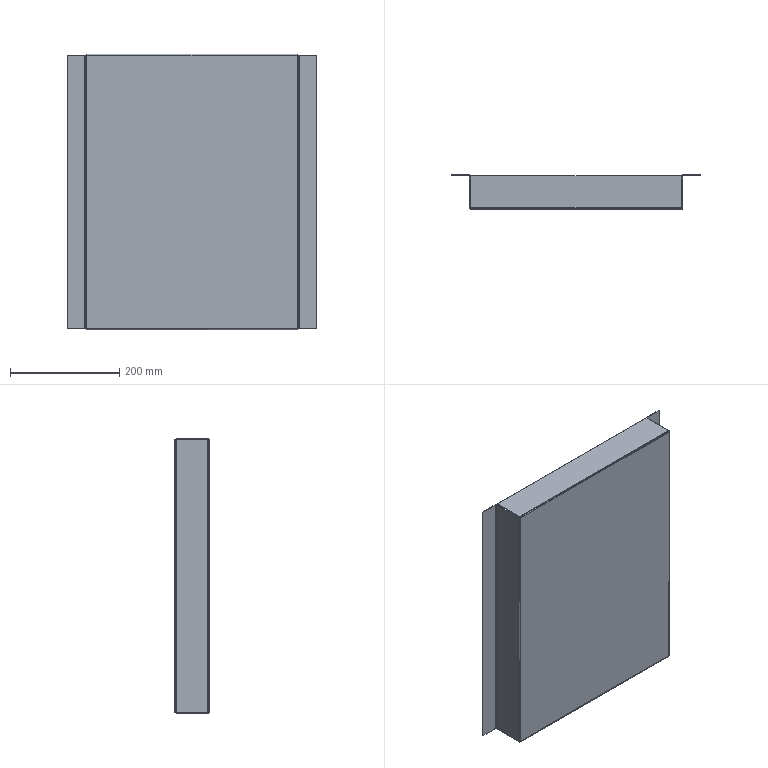Part | SolidWorks | features EdgeFlange 2, FlatPattern 1, SMBaseFlange 1, SheetMetal 1 | 1 solid | 54 faces | box 457 x 62.2 x 504.4 mm | volume 401697 mm3 | plane 34 | cylinder 12 | spline 8 | commonest cylinder face diameters 2 x6 4.4 x6